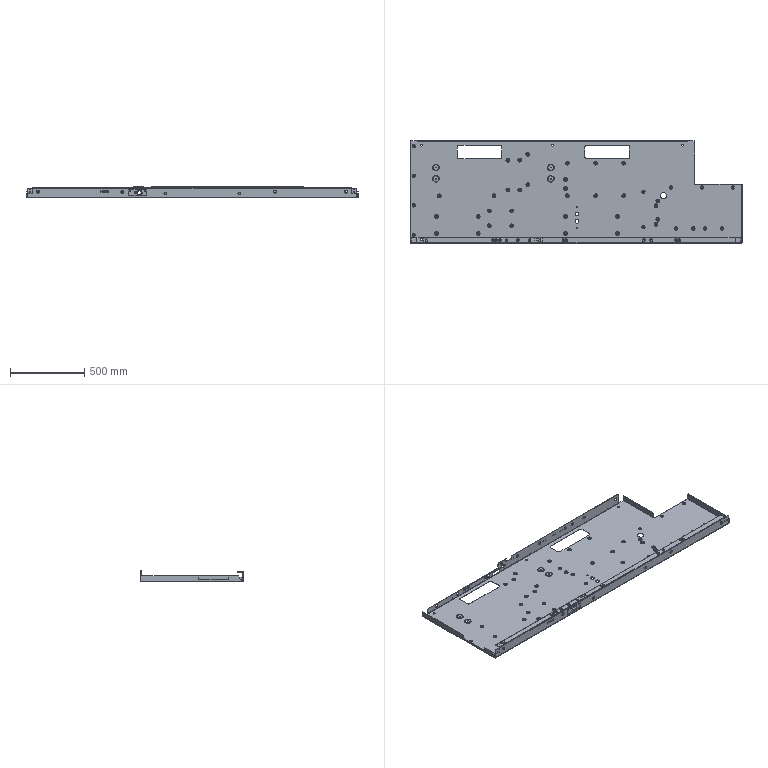Part | STEP file | 1 solid | 1247 faces | box 2240 x 691 x 80 mm | volume 4108988 mm3 | cylinder 429 | plane 422 | torus 392 | spline 4 | commonest cylinder face diameters 4.7 x80 20 x72 24 x72 20.5 x52 18 x30 5.3 x24